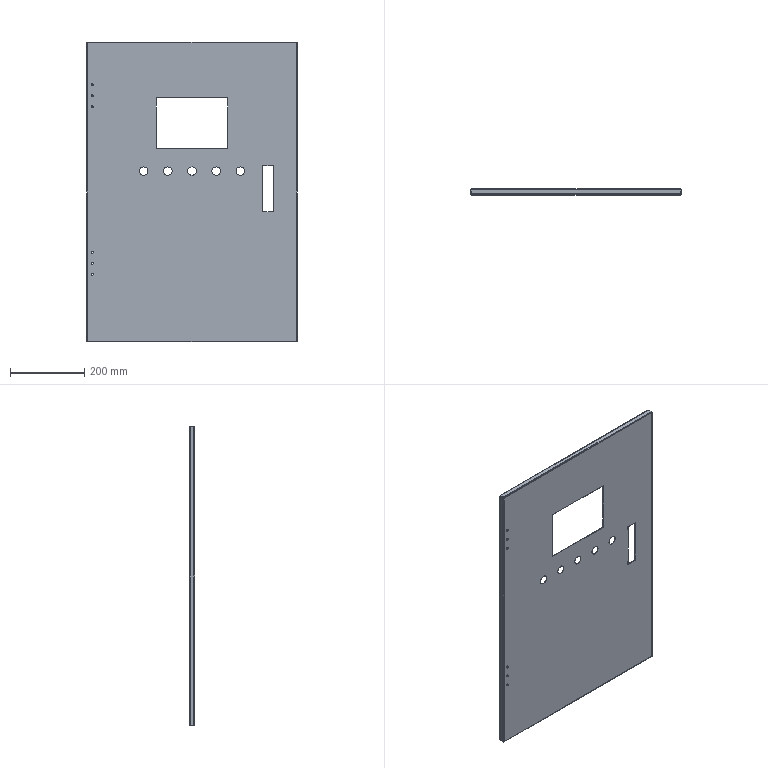Part | SolidWorks | features ICE 3, EdgeFlange 2, Cut 1, FlatPattern 1, LPattern 1, SMBaseFlange 1, SheetMetal 1 | 1 solid | 100 faces | box 566 x 15 x 806 mm | volume 720879 mm3 | plane 46 | cylinder 38 | spline 16 | commonest cylinder face diameters 5.5 x12 23 x10 1.473 x8 4.473 x8